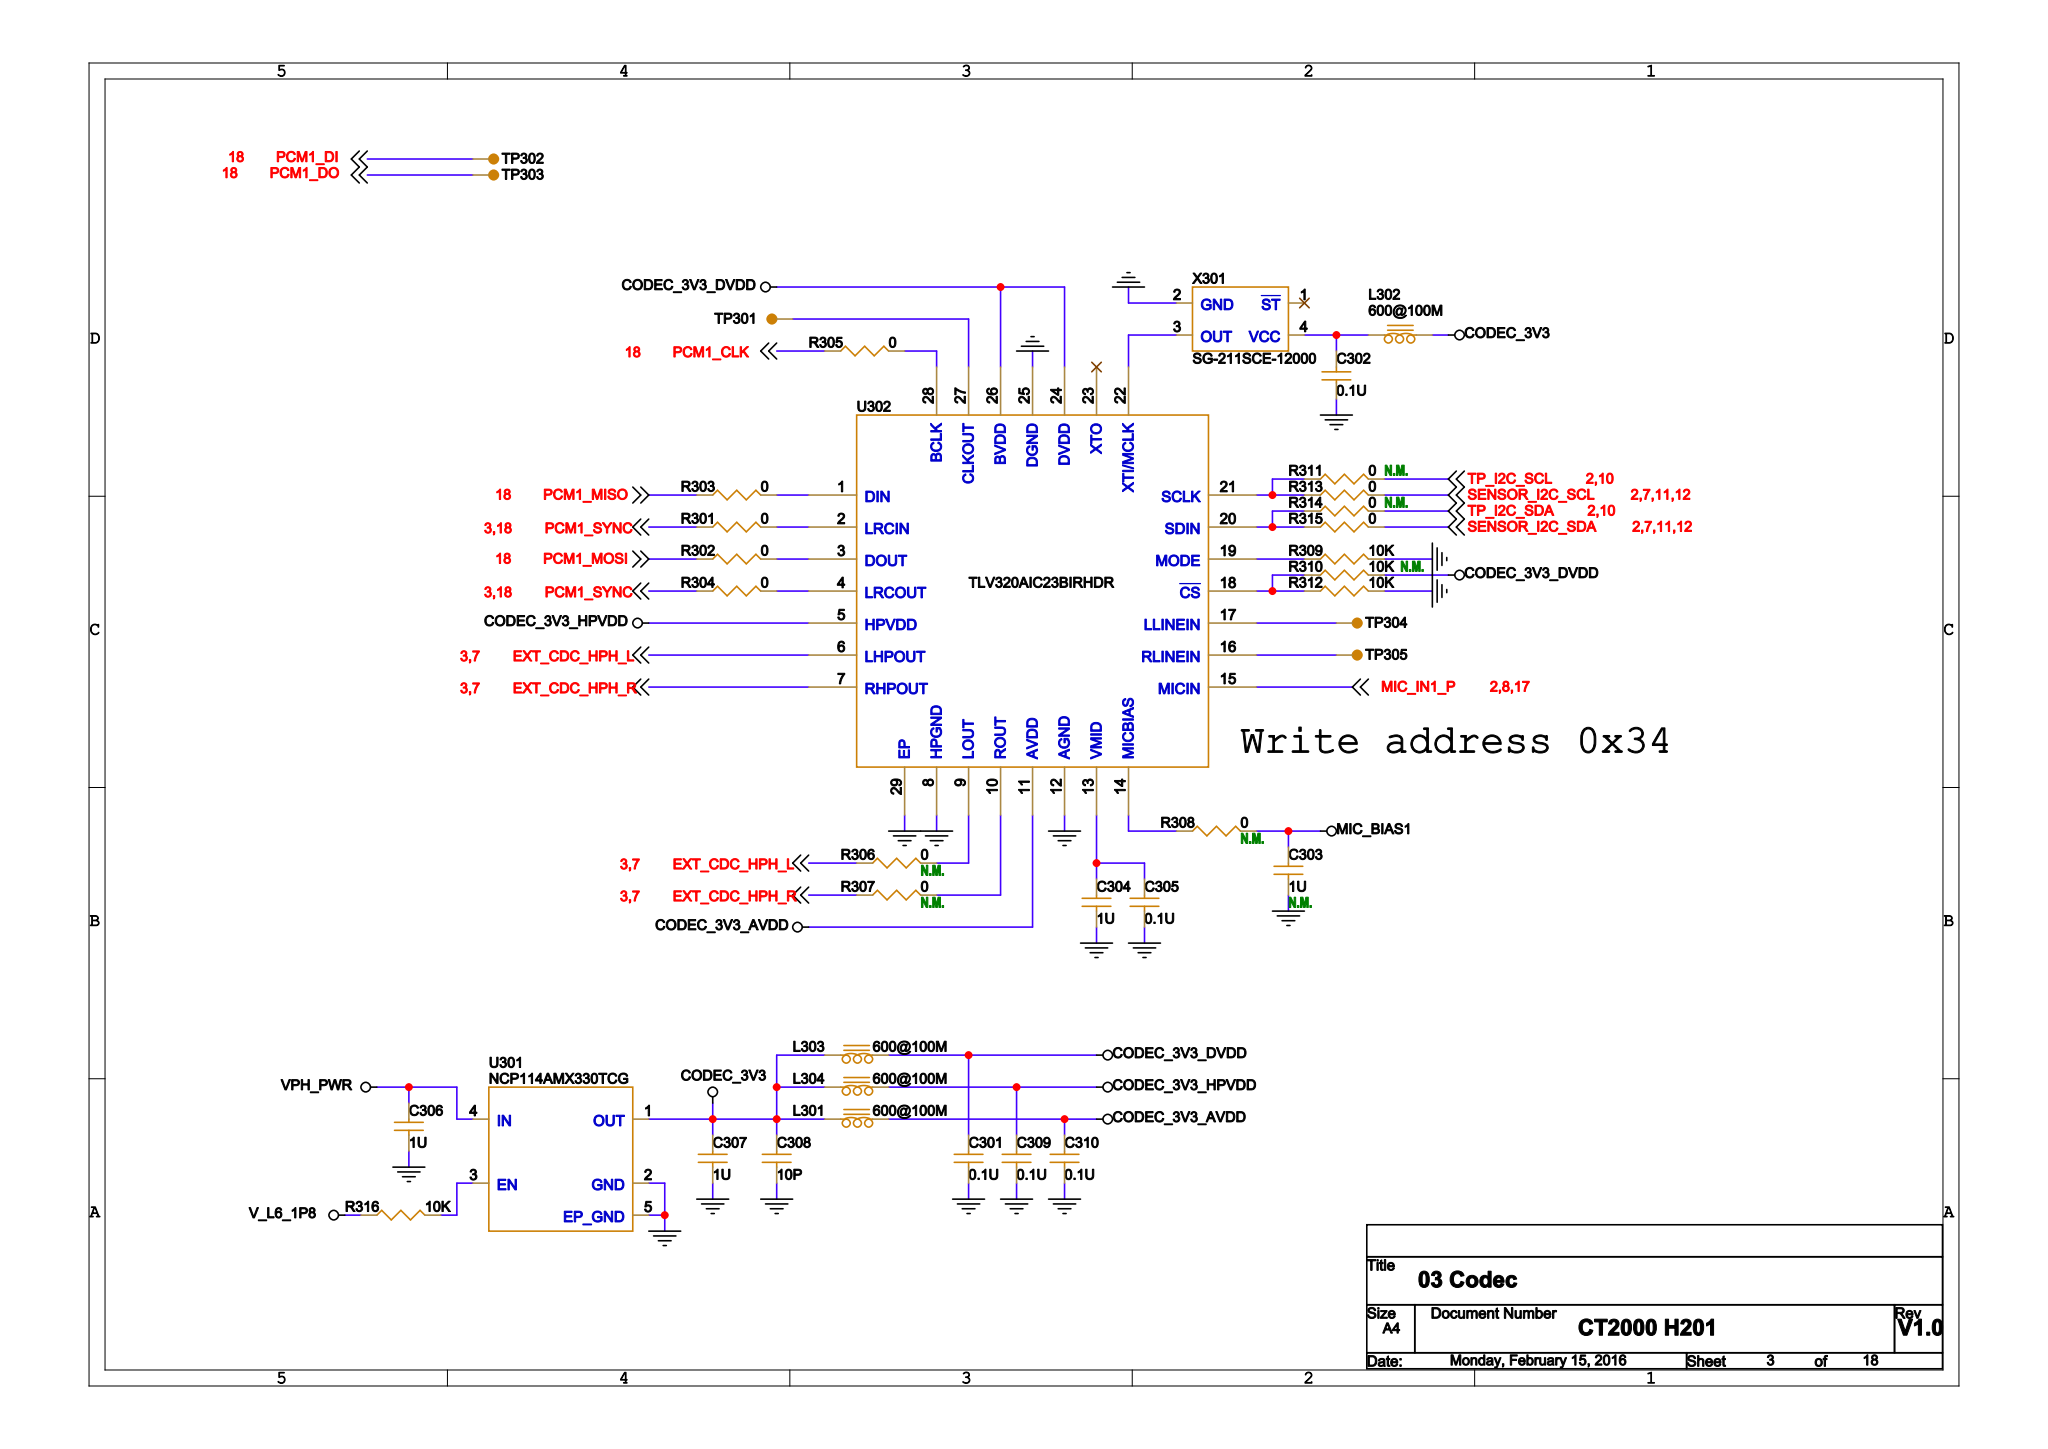Circuit board | Cadence Allegro | 573 parts | 376 nets | one sheet of the schematic
Parts on this sheet (reference | value | footprint):
C301 | 0.1U | C0402
C302 | 0.1U | C0402
C303 | 1U | C0402
C304 | 1U | C0402
C305 | 0.1U | C0402
C306 | 1U | C0402
C307 | 1U | C0402
C308 | 10P | C0402
C309 | 0.1U | C0402
C310 | 0.1U | C0402
L301 | 600@100M | L0402
L302 | 600@100M | L0402
L303 | 600@100M | L0402
L304 | 600@100M | L0402
R301 | 0 | R0402
R302 | 0 | R0402
R303 | 0 | R0402
R304 | 0 | R0402
R305 | 0 | R0402
R306 | 0 | R0402
R307 | 0 | R0402
R308 | 0 | R0402
R309 | 10K | R0402
R310 | 10K | R0402
R311 | 0 | R0402
R312 | 10K | R0402
R313 | 0 | R0402
R314 | 0 | R0402
R315 | 0 | R0402
R316 | 10K | R0402
TP301 | 1 mm | TESTPOINT_32MIL
TP302 | 1 mm | TESTPOINT_32MIL
TP303 | 1 mm | TESTPOINT_32MIL
TP304 | 1 mm | TESTPOINT_32MIL
TP305 | 1 mm | TESTPOINT_32MIL
U301 | NCP114AMX330TCG | UDFN4_1X1X0P7_0P65
U302 | TLV320AIC23BIRHDR | QFN28_5X5X0P9_0P5_EP
X301 | SG-211SCE-12000 | OSC_SG-211SCE-12000
Nets of these parts (net: part-pin ...):
GND: C301-2 C302-1 C303-2 C304-2 C305-2 C306-2 C307-2 C308-2 C309-2 C310-2 R309-2 R312-2 U301-2 U301-5 X301-2 U302-8 U302-12 U302-25 U302-29
CODEC_3V3_AVDD: C310-1 L301-2 U302-11
N52780665: R305-2 U302-28
CODEC_3V3_DVDD: C301-1 L303-2 R310-2 U302-24 U302-26
N52786138: TP301-1 U302-27
N52783850: R310-1 R312-1 U302-18
N52780557: R303-2 U302-1
N52780662: R302-2 U302-3
CODEC_3V3_HPVDD: C309-1 L304-2 U302-5
EXT_CDC_HPH_L: R306-1 U302-6
N52783804: TP304-1 U302-17
N52783170: R306-2 U302-9
N52780577: R301-2 U302-2
N52780580: R304-2 U302-4
N52783435: R308-1 U302-14
MIC_IN1_P: U302-15
N52784028: R309-1 U302-19
EXT_CDC_HPH_R: R307-1 U302-7
N52783796: TP305-1 U302-16
N52783175: R307-2 U302-10
N52784061: R311-1 R313-1 U302-21
N52784064: R314-1 R315-1 U302-20
N52783386: C304-1 C305-1 U302-13
N52786380: X301-3 U302-22
TP_I2C_SDA: R314-2
TP_I2C_SCL: R311-2
MIC_BIAS1: C303-1 R308-2
SENSOR_I2C_SDA: R315-2
VPH_PWR: C306-1 U301-4
SENSOR_I2C_SCL: R313-2
PCM1_MISO: R303-1
PCM1_SYNC: R301-1 R304-1
PCM1_MOSI: R302-1
PCM1_DI: TP302-1
PCM1_DO: TP303-1
PCM1_CLK: R305-1
V_L6_1P8: R316-1
N52822029: C302-2 L302-2 X301-4
CODEC_3V3: C307-1 C308-1 L301-1 L302-1 L303-1 L304-1 U301-1
N52781259: R316-2 U301-3